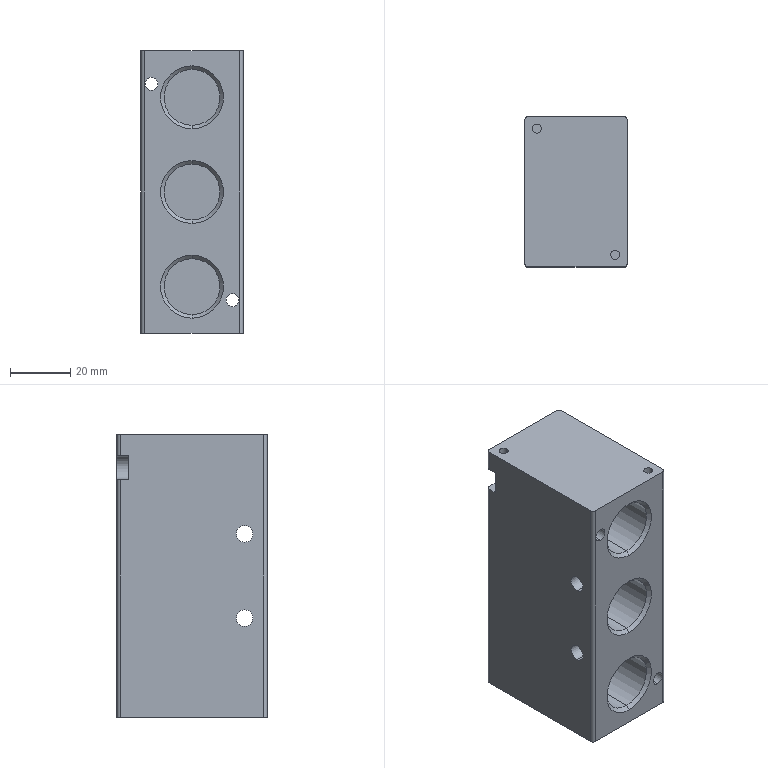Part | STEP file | 4V430C_15_Valve_Body | 1 solid | 65 faces | box 34 x 50 x 94 mm | volume 133275 mm3 | cylinder 34 | plane 21 | cone 10 | commonest cylinder face diameters 18.631 x10 3 x8 2.4 x6 4.3 x4 5.5 x4 8 x2